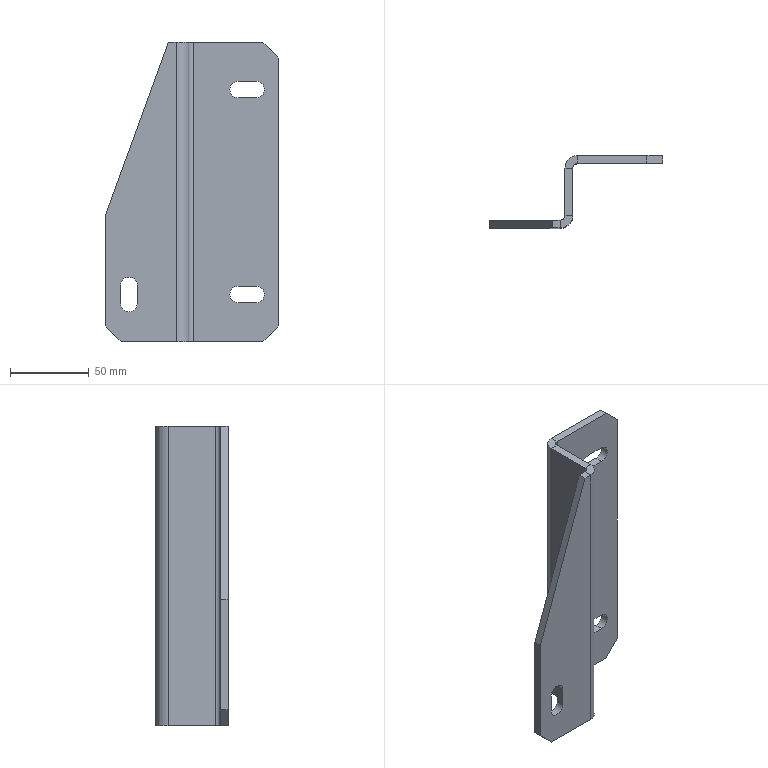Part | STEP file | PRT0001 | 1 solid | 41 faces | box 110 x 46 x 190 mm | volume 124105 mm3 | plane 28 | cylinder 13 | commonest cylinder face diameters 10.5 x9 6 x2 16 x2
STEP:
#1=CARTESIAN_POINT('',(-5.75,0.,124.75));
#2=VERTEX_POINT('',#1);
#3=CARTESIAN_POINT('',(5.75,0.,124.75));
#4=VERTEX_POINT('',#3);
#5=CARTESIAN_POINT('',(-5.75,0.,124.75));
#6=DIRECTION('',(1.,0.,0.));
#7=VECTOR('',#6,1000.);
#8=LINE('',#5,#7);
#9=EDGE_CURVE('',#2,#4,#8,.T.);
#10=ORIENTED_EDGE('',*,*,#9,.F.);
#11=CARTESIAN_POINT('',(-5.75,-5.,124.75));
#12=VERTEX_POINT('',#11);
#13=CARTESIAN_POINT('',(-5.75,-5.,124.75));
#14=DIRECTION('',(0.,1.,0.));
#15=VECTOR('',#14,1000.);
#16=LINE('',#13,#15);
#17=EDGE_CURVE('',#12,#2,#16,.T.);
#18=ORIENTED_EDGE('',*,*,#17,.F.);
#19=CARTESIAN_POINT('',(5.75,-5.,124.75));
#20=VERTEX_POINT('',#19);
#21=CARTESIAN_POINT('',(-5.75,-5.,124.75));
#22=DIRECTION('',(1.,0.,0.));
#23=VECTOR('',#22,1000.);
#24=LINE('',#21,#23);
#25=EDGE_CURVE('',#12,#20,#24,.T.);
#26=ORIENTED_EDGE('',*,*,#25,.T.);
#27=CARTESIAN_POINT('',(5.75,0.,124.75));
#28=DIRECTION('',(0.,-1.,0.));
#29=VECTOR('',#28,1000.);
#30=LINE('',#27,#29);
#31=EDGE_CURVE('',#4,#20,#30,.T.);
#32=ORIENTED_EDGE('',*,*,#31,.F.);
#33=EDGE_LOOP('',(#10,#18,#26,#32));
#34=FACE_OUTER_BOUND('',#33,.T.);
#35=CARTESIAN_POINT('',(-5.75,-10.,124.75));
#36=DIRECTION('',(0.,0.,-1.));
#37=DIRECTION('',(0.,-1.,0.));
#38=AXIS2_PLACEMENT_3D('',#35,#36,#37);
#39=PLANE('',#38);
#40=ADVANCED_FACE('',(#34),#39,.F.);
#41=CARTESIAN_POINT('',(5.75,-5.,135.25));
#42=VERTEX_POINT('',#41);
#43=CARTESIAN_POINT('',(5.75,0.,135.25));
#44=VERTEX_POINT('',#43);
#45=CARTESIAN_POINT('',(5.75,-5.,135.25));
#46=DIRECTION('',(0.,1.,0.));
#47=VECTOR('',#46,1000.);
#48=LINE('',#45,#47);
#49=EDGE_CURVE('',#42,#44,#48,.T.);
#50=ORIENTED_EDGE('',*,*,#49,.T.);
#51=CARTESIAN_POINT('',(5.75,0.,130.));
#52=DIRECTION('',(0.,-1.,0.));
#53=DIRECTION('',(0.,0.,-1.));
#54=AXIS2_PLACEMENT_3D('',#51,#52,#53);
#55=CIRCLE('',#54,5.25);
#56=EDGE_CURVE('',#4,#44,#55,.T.);
#57=ORIENTED_EDGE('',*,*,#56,.F.);
#58=ORIENTED_EDGE('',*,*,#31,.T.);
#59=CARTESIAN_POINT('',(5.75,-5.,130.));
#60=DIRECTION('',(0.,1.,0.));
#61=DIRECTION('',(0.,0.,1.));
#62=AXIS2_PLACEMENT_3D('',#59,#60,#61);
#63=CIRCLE('',#62,5.25);
#64=EDGE_CURVE('',#42,#20,#63,.T.);
#65=ORIENTED_EDGE('',*,*,#64,.F.);
#66=EDGE_LOOP('',(#50,#57,#58,#65));
#67=FACE_OUTER_BOUND('',#66,.T.);
#68=CARTESIAN_POINT('',(5.75,-10.,130.));
#69=DIRECTION('',(0.,1.,0.));
#70=DIRECTION('',(-1.,0.,0.));
#71=AXIS2_PLACEMENT_3D('',#68,#69,#70);
#72=CYLINDRICAL_SURFACE('',#71,5.25);
#73=ADVANCED_FACE('',(#67),#72,.F.);
#74=CARTESIAN_POINT('',(-5.75,0.,135.25));
#75=VERTEX_POINT('',#74);
#76=CARTESIAN_POINT('',(5.75,0.,135.25));
#77=DIRECTION('',(-1.,0.,0.));
#78=VECTOR('',#77,1000.);
#79=LINE('',#76,#78);
#80=EDGE_CURVE('',#44,#75,#79,.T.);
#81=ORIENTED_EDGE('',*,*,#80,.F.);
#82=ORIENTED_EDGE('',*,*,#49,.F.);
#83=CARTESIAN_POINT('',(-5.75,-5.,135.25));
#84=VERTEX_POINT('',#83);
#85=CARTESIAN_POINT('',(5.75,-5.,135.25));
#86=DIRECTION('',(-1.,0.,0.));
#87=VECTOR('',#86,1000.);
#88=LINE('',#85,#87);
#89=EDGE_CURVE('',#42,#84,#88,.T.);
#90=ORIENTED_EDGE('',*,*,#89,.T.);
#91=CARTESIAN_POINT('',(-5.75,0.,135.25));
#92=DIRECTION('',(0.,-1.,0.));
#93=VECTOR('',#92,1000.);
#94=LINE('',#91,#93);
#95=EDGE_CURVE('',#75,#84,#94,.T.);
#96=ORIENTED_EDGE('',*,*,#95,.F.);
#97=EDGE_LOOP('',(#81,#82,#90,#96));
#98=FACE_OUTER_BOUND('',#97,.T.);
#99=CARTESIAN_POINT('',(-5.75,-10.,135.25));
#100=DIRECTION('',(0.,0.,1.));
#101=DIRECTION('',(1.,0.,0.));
#102=AXIS2_PLACEMENT_3D('',#99,#100,#101);
#103=PLANE('',#102);
#104=ADVANCED_FACE('',(#98),#103,.F.);
#105=CARTESIAN_POINT('',(-11.,0.,130.));
#106=VERTEX_POINT('',#105);
#107=CARTESIAN_POINT('',(-11.,-5.,130.));
#108=VERTEX_POINT('',#107);
#109=CARTESIAN_POINT('',(-11.,0.,130.));
#110=DIRECTION('',(0.,-1.,0.));
#111=VECTOR('',#110,1000.);
#112=LINE('',#109,#111);
#113=EDGE_CURVE('',#106,#108,#112,.T.);
#114=ORIENTED_EDGE('',*,*,#113,.F.);
#115=CARTESIAN_POINT('',(-5.75,0.,130.));
#116=DIRECTION('',(0.,-1.,0.));
#117=DIRECTION('',(0.,0.,1.));
#118=AXIS2_PLACEMENT_3D('',#115,#116,#117);
#119=CIRCLE('',#118,5.25);
#120=EDGE_CURVE('',#75,#106,#119,.T.);
#121=ORIENTED_EDGE('',*,*,#120,.F.);
#122=ORIENTED_EDGE('',*,*,#95,.T.);
#123=CARTESIAN_POINT('',(-5.75,-5.,130.));
#124=DIRECTION('',(0.,1.,0.));
#125=DIRECTION('',(-1.,0.,0.));
#126=AXIS2_PLACEMENT_3D('',#123,#124,#125);
#127=CIRCLE('',#126,5.25);
#128=EDGE_CURVE('',#108,#84,#127,.T.);
#129=ORIENTED_EDGE('',*,*,#128,.F.);
#130=EDGE_LOOP('',(#114,#121,#122,#129));
#131=FACE_OUTER_BOUND('',#130,.T.);
#132=CARTESIAN_POINT('',(-5.75,-10.,130.));
#133=DIRECTION('',(0.,1.,0.));
#134=DIRECTION('',(-1.,0.,0.));
#135=AXIS2_PLACEMENT_3D('',#132,#133,#134);
#136=CYLINDRICAL_SURFACE('',#135,5.25);
#137=ADVANCED_FACE('',(#131),#136,.F.);
#138=CARTESIAN_POINT('',(-5.75,-5.,130.));
#139=DIRECTION('',(0.,1.,0.));
#140=DIRECTION('',(0.,0.,-1.));
#141=AXIS2_PLACEMENT_3D('',#138,#139,#140);
#142=CIRCLE('',#141,5.25);
#143=EDGE_CURVE('',#12,#108,#142,.T.);
#144=ORIENTED_EDGE('',*,*,#143,.F.);
#145=ORIENTED_EDGE('',*,*,#17,.T.);
#146=CARTESIAN_POINT('',(-5.75,0.,130.));
#147=DIRECTION('',(0.,-1.,0.));
#148=DIRECTION('',(-1.,0.,0.));
#149=AXIS2_PLACEMENT_3D('',#146,#147,#148);
#150=CIRCLE('',#149,5.25);
#151=EDGE_CURVE('',#106,#2,#150,.T.);
#152=ORIENTED_EDGE('',*,*,#151,.F.);
#153=ORIENTED_EDGE('',*,*,#113,.T.);
#154=EDGE_LOOP('',(#144,#145,#152,#153));
#155=FACE_OUTER_BOUND('',#154,.T.);
#156=CARTESIAN_POINT('',(-5.75,-10.,130.));
#157=DIRECTION('',(0.,1.,0.));
#158=DIRECTION('',(-1.,0.,0.));
#159=AXIS2_PLACEMENT_3D('',#156,#157,#158);
#160=CYLINDRICAL_SURFACE('',#159,5.25);
#161=ADVANCED_FACE('',(#155),#160,.F.);
#162=CARTESIAN_POINT('',(-5.75,0.,-5.25));
#163=VERTEX_POINT('',#162);
#164=CARTESIAN_POINT('',(5.75,0.,-5.25));
#165=VERTEX_POINT('',#164);
#166=CARTESIAN_POINT('',(-5.75,0.,-5.25));
#167=DIRECTION('',(1.,0.,0.));
#168=VECTOR('',#167,1000.);
#169=LINE('',#166,#168);
#170=EDGE_CURVE('',#163,#165,#169,.T.);
#171=ORIENTED_EDGE('',*,*,#170,.F.);
#172=CARTESIAN_POINT('',(-5.75,-5.,-5.25));
#173=VERTEX_POINT('',#172);
#174=CARTESIAN_POINT('',(-5.75,-5.,-5.25));
#175=DIRECTION('',(0.,1.,0.));
#176=VECTOR('',#175,1000.);
#177=LINE('',#174,#176);
#178=EDGE_CURVE('',#173,#163,#177,.T.);
#179=ORIENTED_EDGE('',*,*,#178,.F.);
#180=CARTESIAN_POINT('',(5.75,-5.,-5.25));
#181=VERTEX_POINT('',#180);
#182=CARTESIAN_POINT('',(-5.75,-5.,-5.25));
#183=DIRECTION('',(1.,0.,0.));
#184=VECTOR('',#183,1000.);
#185=LINE('',#182,#184);
#186=EDGE_CURVE('',#173,#181,#185,.T.);
#187=ORIENTED_EDGE('',*,*,#186,.T.);
#188=CARTESIAN_POINT('',(5.75,0.,-5.25));
#189=DIRECTION('',(0.,-1.,0.));
#190=VECTOR('',#189,1000.);
#191=LINE('',#188,#190);
#192=EDGE_CURVE('',#165,#181,#191,.T.);
#193=ORIENTED_EDGE('',*,*,#192,.F.);
#194=EDGE_LOOP('',(#171,#179,#187,#193));
#195=FACE_OUTER_BOUND('',#194,.T.);
#196=CARTESIAN_POINT('',(-5.75,-10.,-5.25));
#197=DIRECTION('',(0.,0.,-1.));
#198=DIRECTION('',(0.,-1.,0.));
#199=AXIS2_PLACEMENT_3D('',#196,#197,#198);
#200=PLANE('',#199);
#201=ADVANCED_FACE('',(#195),#200,.F.);
#202=CARTESIAN_POINT('',(5.75,-5.,5.25));
#203=VERTEX_POINT('',#202);
#204=CARTESIAN_POINT('',(5.75,0.,5.25));
#205=VERTEX_POINT('',#204);
#206=CARTESIAN_POINT('',(5.75,-5.,5.25));
#207=DIRECTION('',(0.,1.,0.));
#208=VECTOR('',#207,1000.);
#209=LINE('',#206,#208);
#210=EDGE_CURVE('',#203,#205,#209,.T.);
#211=ORIENTED_EDGE('',*,*,#210,.T.);
#212=CARTESIAN_POINT('',(5.75,0.,0.));
#213=DIRECTION('',(0.,-1.,0.));
#214=DIRECTION('',(0.,0.,-1.));
#215=AXIS2_PLACEMENT_3D('',#212,#213,#214);
#216=CIRCLE('',#215,5.25);
#217=EDGE_CURVE('',#165,#205,#216,.T.);
#218=ORIENTED_EDGE('',*,*,#217,.F.);
#219=ORIENTED_EDGE('',*,*,#192,.T.);
#220=CARTESIAN_POINT('',(5.75,-5.,0.));
#221=DIRECTION('',(0.,1.,0.));
#222=DIRECTION('',(0.,0.,1.));
#223=AXIS2_PLACEMENT_3D('',#220,#221,#222);
#224=CIRCLE('',#223,5.25);
#225=EDGE_CURVE('',#203,#181,#224,.T.);
#226=ORIENTED_EDGE('',*,*,#225,.F.);
#227=EDGE_LOOP('',(#211,#218,#219,#226));
#228=FACE_OUTER_BOUND('',#227,.T.);
#229=CARTESIAN_POINT('',(5.75,-10.,0.));
#230=DIRECTION('',(0.,1.,0.));
#231=DIRECTION('',(-1.,0.,0.));
#232=AXIS2_PLACEMENT_3D('',#229,#230,#231);
#233=CYLINDRICAL_SURFACE('',#232,5.25);
#234=ADVANCED_FACE('',(#228),#233,.F.);
#235=CARTESIAN_POINT('',(-5.75,0.,5.25));
#236=VERTEX_POINT('',#235);
#237=CARTESIAN_POINT('',(5.75,0.,5.25));
#238=DIRECTION('',(-1.,0.,0.));
#239=VECTOR('',#238,1000.);
#240=LINE('',#237,#239);
#241=EDGE_CURVE('',#205,#236,#240,.T.);
#242=ORIENTED_EDGE('',*,*,#241,.F.);
#243=ORIENTED_EDGE('',*,*,#210,.F.);
#244=CARTESIAN_POINT('',(-5.75,-5.,5.25));
#245=VERTEX_POINT('',#244);
#246=CARTESIAN_POINT('',(5.75,-5.,5.25));
#247=DIRECTION('',(-1.,0.,0.));
#248=VECTOR('',#247,1000.);
#249=LINE('',#246,#248);
#250=EDGE_CURVE('',#203,#245,#249,.T.);
#251=ORIENTED_EDGE('',*,*,#250,.T.);
#252=CARTESIAN_POINT('',(-5.75,0.,5.25));
#253=DIRECTION('',(0.,-1.,0.));
#254=VECTOR('',#253,1000.);
#255=LINE('',#252,#254);
#256=EDGE_CURVE('',#236,#245,#255,.T.);
#257=ORIENTED_EDGE('',*,*,#256,.F.);
#258=EDGE_LOOP('',(#242,#243,#251,#257));
#259=FACE_OUTER_BOUND('',#258,.T.);
#260=CARTESIAN_POINT('',(-5.75,-10.,5.25));
#261=DIRECTION('',(0.,0.,1.));
#262=DIRECTION('',(1.,0.,0.));
#263=AXIS2_PLACEMENT_3D('',#260,#261,#262);
#264=PLANE('',#263);
#265=ADVANCED_FACE('',(#259),#264,.F.);
#266=CARTESIAN_POINT('',(-11.,0.,0.));
#267=VERTEX_POINT('',#266);
#268=CARTESIAN_POINT('',(-11.,-5.,0.));
#269=VERTEX_POINT('',#268);
#270=CARTESIAN_POINT('',(-11.,0.,0.));
#271=DIRECTION('',(0.,-1.,0.));
#272=VECTOR('',#271,1000.);
#273=LINE('',#270,#272);
#274=EDGE_CURVE('',#267,#269,#273,.T.);
#275=ORIENTED_EDGE('',*,*,#274,.F.);
#276=CARTESIAN_POINT('',(-5.75,0.,0.));
#277=DIRECTION('',(0.,-1.,0.));
#278=DIRECTION('',(0.,0.,1.));
#279=AXIS2_PLACEMENT_3D('',#276,#277,#278);
#280=CIRCLE('',#279,5.25);
#281=EDGE_CURVE('',#236,#267,#280,.T.);
#282=ORIENTED_EDGE('',*,*,#281,.F.);
#283=ORIENTED_EDGE('',*,*,#256,.T.);
#284=CARTESIAN_POINT('',(-5.75,-5.,0.));
#285=DIRECTION('',(0.,1.,0.));
#286=DIRECTION('',(-1.,0.,0.));
#287=AXIS2_PLACEMENT_3D('',#284,#285,#286);
#288=CIRCLE('',#287,5.25);
#289=EDGE_CURVE('',#269,#245,#288,.T.);
#290=ORIENTED_EDGE('',*,*,#289,.F.);
#291=EDGE_LOOP('',(#275,#282,#283,#290));
#292=FACE_OUTER_BOUND('',#291,.T.);
#293=CARTESIAN_POINT('',(-5.75,-10.,0.));
#294=DIRECTION('',(0.,1.,0.));
#295=DIRECTION('',(-1.,0.,0.));
#296=AXIS2_PLACEMENT_3D('',#293,#294,#295);
#297=CYLINDRICAL_SURFACE('',#296,5.25);
#298=ADVANCED_FACE('',(#292),#297,.F.);
#299=CARTESIAN_POINT('',(-5.75,-5.,0.));
#300=DIRECTION('',(0.,1.,0.));
#301=DIRECTION('',(0.,0.,-1.));
#302=AXIS2_PLACEMENT_3D('',#299,#300,#301);
#303=CIRCLE('',#302,5.25);
#304=EDGE_CURVE('',#173,#269,#303,.T.);
#305=ORIENTED_EDGE('',*,*,#304,.F.);
#306=ORIENTED_EDGE('',*,*,#178,.T.);
#307=CARTESIAN_POINT('',(-5.75,0.,0.));
#308=DIRECTION('',(0.,-1.,0.));
#309=DIRECTION('',(-1.,0.,0.));
#310=AXIS2_PLACEMENT_3D('',#307,#308,#309);
#311=CIRCLE('',#310,5.25);
#312=EDGE_CURVE('',#267,#163,#311,.T.);
#313=ORIENTED_EDGE('',*,*,#312,.F.);
#314=ORIENTED_EDGE('',*,*,#274,.T.);
#315=EDGE_LOOP('',(#305,#306,#313,#314));
#316=FACE_OUTER_BOUND('',#315,.T.);
#317=CARTESIAN_POINT('',(-5.75,-10.,0.));
#318=DIRECTION('',(0.,1.,0.));
#319=DIRECTION('',(-1.,0.,0.));
#320=AXIS2_PLACEMENT_3D('',#317,#318,#319);
#321=CYLINDRICAL_SURFACE('',#320,5.25);
#322=ADVANCED_FACE('',(#316),#321,.F.);
#323=CARTESIAN_POINT('',(20.,0.,-20.));
#324=VERTEX_POINT('',#323);
#325=CARTESIAN_POINT('',(20.,-5.,-20.));
#326=VERTEX_POINT('',#325);
#327=CARTESIAN_POINT('',(20.,0.,-20.));
#328=DIRECTION('',(0.,-1.,0.));
#329=VECTOR('',#328,1000.);
#330=LINE('',#327,#329);
#331=EDGE_CURVE('',#324,#326,#330,.T.);
#332=ORIENTED_EDGE('',*,*,#331,.T.);
#333=CARTESIAN_POINT('',(10.,-5.,-30.));
#334=VERTEX_POINT('',#333);
#335=CARTESIAN_POINT('',(10.,-5.,-30.));
#336=DIRECTION('',(0.7071,0.,0.7071));
#337=VECTOR('',#336,1000.);
#338=LINE('',#335,#337);
#339=EDGE_CURVE('',#334,#326,#338,.T.);
#340=ORIENTED_EDGE('',*,*,#339,.F.);
#341=CARTESIAN_POINT('',(10.,0.,-30.));
#342=VERTEX_POINT('',#341);
#343=CARTESIAN_POINT('',(10.,-5.,-30.));
#344=DIRECTION('',(0.,1.,0.));
#345=VECTOR('',#344,1000.);
#346=LINE('',#343,#345);
#347=EDGE_CURVE('',#334,#342,#346,.T.);
#348=ORIENTED_EDGE('',*,*,#347,.T.);
#349=CARTESIAN_POINT('',(20.,0.,-20.));
#350=DIRECTION('',(-0.7071,0.,-0.7071));
#351=VECTOR('',#350,1000.);
#352=LINE('',#349,#351);
#353=EDGE_CURVE('',#324,#342,#352,.T.);
#354=ORIENTED_EDGE('',*,*,#353,.F.);
#355=EDGE_LOOP('',(#332,#340,#348,#354));
#356=FACE_OUTER_BOUND('',#355,.T.);
#357=CARTESIAN_POINT('',(10.,-8.,-30.));
#358=DIRECTION('',(0.7071,0.,-0.7071));
#359=DIRECTION('',(0.,-1.,0.));
#360=AXIS2_PLACEMENT_3D('',#357,#358,#359);
#361=PLANE('',#360);
#362=ADVANCED_FACE('',(#356),#361,.T.);
#363=CARTESIAN_POINT('',(-80.25,-41.,5.75));
#364=VERTEX_POINT('',#363);
#365=CARTESIAN_POINT('',(-80.25,-41.,-5.75));
#366=VERTEX_POINT('',#365);
#367=CARTESIAN_POINT('',(-80.25,-41.,5.75));
#368=DIRECTION('',(0.,0.,-1.));
#369=VECTOR('',#368,1000.);
#370=LINE('',#367,#369);
#371=EDGE_CURVE('',#364,#366,#370,.T.);
#372=ORIENTED_EDGE('',*,*,#371,.F.);
#373=CARTESIAN_POINT('',(-80.25,-46.,5.75));
#374=VERTEX_POINT('',#373);
#375=CARTESIAN_POINT('',(-80.25,-46.,5.75));
#376=DIRECTION('',(0.,1.,0.));
#377=VECTOR('',#376,1000.);
#378=LINE('',#375,#377);
#379=EDGE_CURVE('',#374,#364,#378,.T.);
#380=ORIENTED_EDGE('',*,*,#379,.F.);
#381=CARTESIAN_POINT('',(-80.25,-46.,-5.75));
#382=VERTEX_POINT('',#381);
#383=CARTESIAN_POINT('',(-80.25,-46.,5.75));
#384=DIRECTION('',(0.,0.,-1.));
#385=VECTOR('',#384,1000.);
#386=LINE('',#383,#385);
#387=EDGE_CURVE('',#374,#382,#386,.T.);
#388=ORIENTED_EDGE('',*,*,#387,.T.);
#389=CARTESIAN_POINT('',(-80.25,-41.,-5.75));
#390=DIRECTION('',(0.,-1.,0.));
#391=VECTOR('',#390,1000.);
#392=LINE('',#389,#391);
#393=EDGE_CURVE('',#366,#382,#392,.T.);
#394=ORIENTED_EDGE('',*,*,#393,.F.);
#395=EDGE_LOOP('',(#372,#380,#388,#394));
#396=FACE_OUTER_BOUND('',#395,.T.);
#397=CARTESIAN_POINT('',(-80.25,-51.,5.75));
#398=DIRECTION('',(-1.,0.,0.));
#399=DIRECTION('',(0.,0.,1.));
#400=AXIS2_PLACEMENT_3D('',#397,#398,#399);
#401=PLANE('',#400);
#402=ADVANCED_FACE('',(#396),#401,.F.);
#403=CARTESIAN_POINT('',(-69.75,-46.,-5.75));
#404=VERTEX_POINT('',#403);
#405=CARTESIAN_POINT('',(-69.75,-41.,-5.75));
#406=VERTEX_POINT('',#405);
#407=CARTESIAN_POINT('',(-69.75,-46.,-5.75));
#408=DIRECTION('',(0.,1.,0.));
#409=VECTOR('',#408,1000.);
#410=LINE('',#407,#409);
#411=EDGE_CURVE('',#404,#406,#410,.T.);
#412=ORIENTED_EDGE('',*,*,#411,.T.);
#413=CARTESIAN_POINT('',(-75.,-41.,-5.75));
#414=DIRECTION('',(0.,-1.,0.));
#415=DIRECTION('',(-1.,0.,0.));
#416=AXIS2_PLACEMENT_3D('',#413,#414,#415);
#417=CIRCLE('',#416,5.25);
#418=EDGE_CURVE('',#366,#406,#417,.T.);
#419=ORIENTED_EDGE('',*,*,#418,.F.);
#420=ORIENTED_EDGE('',*,*,#393,.T.);
#421=CARTESIAN_POINT('',(-75.,-46.,-5.75));
#422=DIRECTION('',(0.,1.,0.));
#423=DIRECTION('',(1.,0.,0.));
#424=AXIS2_PLACEMENT_3D('',#421,#422,#423);
#425=CIRCLE('',#424,5.25);
#426=EDGE_CURVE('',#404,#382,#425,.T.);
#427=ORIENTED_EDGE('',*,*,#426,.F.);
#428=EDGE_LOOP('',(#412,#419,#420,#427));
#429=FACE_OUTER_BOUND('',#428,.T.);
#430=CARTESIAN_POINT('',(-75.,-51.,-5.75));
#431=DIRECTION('',(0.,1.,0.));
#432=DIRECTION('',(0.,0.,1.));
#433=AXIS2_PLACEMENT_3D('',#430,#431,#432);
#434=CYLINDRICAL_SURFACE('',#433,5.25);
#435=ADVANCED_FACE('',(#429),#434,.F.);
#436=CARTESIAN_POINT('',(-69.75,-41.,5.75));
#437=VERTEX_POINT('',#436);
#438=CARTESIAN_POINT('',(-69.75,-41.,-5.75));
#439=DIRECTION('',(0.,0.,1.));
#440=VECTOR('',#439,1000.);
#441=LINE('',#438,#440);
#442=EDGE_CURVE('',#406,#437,#441,.T.);
#443=ORIENTED_EDGE('',*,*,#442,.F.);
#444=ORIENTED_EDGE('',*,*,#411,.F.);
#445=CARTESIAN_POINT('',(-69.75,-46.,5.75));
#446=VERTEX_POINT('',#445);
#447=CARTESIAN_POINT('',(-69.75,-46.,-5.75));
#448=DIRECTION('',(0.,0.,1.));
#449=VECTOR('',#448,1000.);
#450=LINE('',#447,#449);
#451=EDGE_CURVE('',#404,#446,#450,.T.);
#452=ORIENTED_EDGE('',*,*,#451,.T.);
#453=CARTESIAN_POINT('',(-69.75,-41.,5.75));
#454=DIRECTION('',(0.,-1.,0.));
#455=VECTOR('',#454,1000.);
#456=LINE('',#453,#455);
#457=EDGE_CURVE('',#437,#446,#456,.T.);
#458=ORIENTED_EDGE('',*,*,#457,.F.);
#459=EDGE_LOOP('',(#443,#444,#452,#458));
#460=FACE_OUTER_BOUND('',#459,.T.);
#461=CARTESIAN_POINT('',(-69.75,-51.,5.75));
#462=DIRECTION('',(1.,0.,0.));
#463=DIRECTION('',(0.,1.,0.));
#464=AXIS2_PLACEMENT_3D('',#461,#462,#463);
#465=PLANE('',#464);
#466=ADVANCED_FACE('',(#460),#465,.F.);
#467=CARTESIAN_POINT('',(-75.,-41.,11.));
#468=VERTEX_POINT('',#467);
#469=CARTESIAN_POINT('',(-75.,-46.,11.));
#470=VERTEX_POINT('',#469);
#471=CARTESIAN_POINT('',(-75.,-41.,11.));
#472=DIRECTION('',(0.,-1.,0.));
#473=VECTOR('',#472,1000.);
#474=LINE('',#471,#473);
#475=EDGE_CURVE('',#468,#470,#474,.T.);
#476=ORIENTED_EDGE('',*,*,#475,.F.);
#477=CARTESIAN_POINT('',(-75.,-41.,5.75));
#478=DIRECTION('',(0.,-1.,0.));
#479=DIRECTION('',(1.,0.,0.));
#480=AXIS2_PLACEMENT_3D('',#477,#478,#479);
#481=CIRCLE('',#480,5.25);
#482=EDGE_CURVE('',#437,#468,#481,.T.);
#483=ORIENTED_EDGE('',*,*,#482,.F.);
#484=ORIENTED_EDGE('',*,*,#457,.T.);
#485=CARTESIAN_POINT('',(-75.,-46.,5.75));
#486=DIRECTION('',(0.,1.,0.));
#487=DIRECTION('',(0.,0.,1.));
#488=AXIS2_PLACEMENT_3D('',#485,#486,#487);
#489=CIRCLE('',#488,5.25);
#490=EDGE_CURVE('',#470,#446,#489,.T.);
#491=ORIENTED_EDGE('',*,*,#490,.F.);
#492=EDGE_LOOP('',(#476,#483,#484,#491));
#493=FACE_OUTER_BOUND('',#492,.T.);
#494=CARTESIAN_POINT('',(-75.,-51.,5.75));
#495=DIRECTION('',(0.,1.,0.));
#496=DIRECTION('',(0.,0.,1.));
#497=AXIS2_PLACEMENT_3D('',#494,#495,#496);
#498=CYLINDRICAL_SURFACE('',#497,5.25);
#499=ADVANCED_FACE('',(#493),#498,.F.);
#500=CARTESIAN_POINT('',(-75.,-46.,5.75));
#501=DIRECTION('',(0.,1.,0.));
#502=DIRECTION('',(-1.,0.,0.));
#503=AXIS2_PLACEMENT_3D('',#500,#501,#502);
#504=CIRCLE('',#503,5.25);
#505=EDGE_CURVE('',#374,#470,#504,.T.);
#506=ORIENTED_EDGE('',*,*,#505,.F.);
#507=ORIENTED_EDGE('',*,*,#379,.T.);
#508=CARTESIAN_POINT('',(-75.,-41.,5.75));
#509=DIRECTION('',(0.,-1.,0.));
#510=DIRECTION('',(0.,0.,1.));
#511=AXIS2_PLACEMENT_3D('',#508,#509,#510);
#512=CIRCLE('',#511,5.25);
#513=EDGE_CURVE('',#468,#364,#512,.T.);
#514=ORIENTED_EDGE('',*,*,#513,.F.);
#515=ORIENTED_EDGE('',*,*,#475,.T.);
#516=EDGE_LOOP('',(#506,#507,#514,#515));
#517=FACE_OUTER_BOUND('',#516,.T.);
#518=CARTESIAN_POINT('',(-75.,-51.,5.75));
#519=DIRECTION('',(0.,1.,0.));
#520=DIRECTION('',(0.,0.,1.));
#521=AXIS2_PLACEMENT_3D('',#518,#519,#520);
#522=CYLINDRICAL_SURFACE('',#521,5.25);
#523=ADVANCED_FACE('',(#517),#522,.F.);
#524=CARTESIAN_POINT('',(-90.,-46.,-20.));
#525=VERTEX_POINT('',#524);
#526=CARTESIAN_POINT('',(-90.,-41.,-20.));
#527=VERTEX_POINT('',#526);
#528=CARTESIAN_POINT('',(-90.,-46.,-20.));
#529=DIRECTION('',(0.,1.,0.));
#530=VECTOR('',#529,1000.);
#531=LINE('',#528,#530);
#532=EDGE_CURVE('',#525,#527,#531,.T.);
#533=ORIENTED_EDGE('',*,*,#532,.T.);
#534=CARTESIAN_POINT('',(-80.,-41.,-30.));
#535=VERTEX_POINT('',#534);
#536=CARTESIAN_POINT('',(-80.,-41.,-30.));
#537=DIRECTION('',(-0.7071,0.,0.7071));
#538=VECTOR('',#537,1000.);
#539=LINE('',#536,#538);
#540=EDGE_CURVE('',#535,#527,#539,.T.);
#541=ORIENTED_EDGE('',*,*,#540,.F.);
#542=CARTESIAN_POINT('',(-80.,-46.,-30.));
#543=VERTEX_POINT('',#542);
#544=CARTESIAN_POINT('',(-80.,-41.,-30.));
#545=DIRECTION('',(0.,-1.,0.));
#546=VECTOR('',#545,1000.);
#547=LINE('',#544,#546);
#548=EDGE_CURVE('',#535,#543,#547,.T.);
#549=ORIENTED_EDGE('',*,*,#548,.T.);
#550=CARTESIAN_POINT('',(-90.,-46.,-20.));
#551=DIRECTION('',(0.7071,0.,-0.7071));
#552=VECTOR('',#551,1000.);
#553=LINE('',#550,#552);
#554=EDGE_CURVE('',#525,#543,#553,.T.);
#555=ORIENTED_EDGE('',*,*,#554,.F.);
#556=EDGE_LOOP('',(#533,#541,#549,#555));
#557=FACE_OUTER_BOUND('',#556,.T.);
#558=CARTESIAN_POINT('',(-80.,-38.,-30.));
#559=DIRECTION('',(0.7071,0.,0.7071));
#560=DIRECTION('',(0.,-1.,0.));
#561=AXIS2_PLACEMENT_3D('',#558,#559,#560);
#562=PLANE('',#561);
#563=ADVANCED_FACE('',(#557),#562,.F.);
#564=CARTESIAN_POINT('',(-90.,-41.,50.));
#565=VERTEX_POINT('',#564);
#566=CARTESIAN_POINT('',(-90.,-41.,-20.));
#567=DIRECTION('',(0.,0.,1.));
#568=VECTOR('',#567,1000.);
#569=LINE('',#566,#568);
#570=EDGE_CURVE('',#527,#565,#569,.T.);
#571=ORIENTED_EDGE('',*,*,#570,.F.);
#572=ORIENTED_EDGE('',*,*,#532,.F.);
#573=CARTESIAN_POINT('',(-90.,-46.,50.));
#574=VERTEX_POINT('',#573);
#575=CARTESIAN_POINT('',(-90.,-46.,-20.));
#576=DIRECTION('',(0.,0.,1.));
#577=VECTOR('',#576,1000.);
#578=LINE('',#575,#577);
#579=EDGE_CURVE('',#525,#574,#578,.T.);
#580=ORIENTED_EDGE('',*,*,#579,.T.);
#581=CARTESIAN_POINT('',(-90.,-41.,50.));
#582=DIRECTION('',(0.,-1.,0.));
#583=VECTOR('',#582,1000.);
#584=LINE('',#581,#583);
#585=EDGE_CURVE('',#565,#574,#584,.T.);
#586=ORIENTED_EDGE('',*,*,#585,.F.);
#587=EDGE_LOOP('',(#571,#572,#580,#586));
#588=FACE_OUTER_BOUND('',#587,.T.);
#589=CARTESIAN_POINT('',(-90.,-46.,160.));
#590=DIRECTION('',(-1.,0.,0.));
#591=DIRECTION('',(0.,0.,1.));
#592=AXIS2_PLACEMENT_3D('',#589,#590,#591);
#593=PLANE('',#592);
#594=ADVANCED_FACE('',(#588),#593,.T.);
#595=ORIENTED_EDGE('',*,*,#371,.T.);
#596=ORIENTED_EDGE('',*,*,#418,.T.);
#597=ORIENTED_EDGE('',*,*,#442,.T.);
#598=ORIENTED_EDGE('',*,*,#482,.T.);
#599=ORIENTED_EDGE('',*,*,#513,.T.);
#600=EDGE_LOOP('',(#595,#596,#597,#598,#599));
#601=FACE_BOUND('',#600,.T.);
#602=CARTESIAN_POINT('',(-45.,-41.,160.));
#603=VERTEX_POINT('',#602);
#604=CARTESIAN_POINT('',(-50.,-41.,160.));
#605=VERTEX_POINT('',#604);
#606=CARTESIAN_POINT('',(-45.,-41.,160.));
#607=DIRECTION('',(-1.,0.,0.));
#608=VECTOR('',#607,1000.);
#609=LINE('',#606,#608);
#610=EDGE_CURVE('',#603,#605,#609,.T.);
#611=ORIENTED_EDGE('',*,*,#610,.F.);
#612=CARTESIAN_POINT('',(-45.,-41.,-30.));
#613=VERTEX_POINT('',#612);
#614=CARTESIAN_POINT('',(-45.,-41.,-30.));
#615=DIRECTION('',(0.,0.,1.));
#616=VECTOR('',#615,1000.);
#617=LINE('',#614,#616);
#618=EDGE_CURVE('',#613,#603,#617,.T.);
#619=ORIENTED_EDGE('',*,*,#618,.F.);
#620=CARTESIAN_POINT('',(-45.,-41.,-30.));
#621=DIRECTION('',(-1.,0.,0.));
#622=VECTOR('',#621,1000.);
#623=LINE('',#620,#622);
#624=EDGE_CURVE('',#613,#535,#623,.T.);
#625=ORIENTED_EDGE('',*,*,#624,.T.);
#626=ORIENTED_EDGE('',*,*,#540,.T.);
#627=ORIENTED_EDGE('',*,*,#570,.T.);
#628=CARTESIAN_POINT('',(-90.,-41.,50.));
#629=DIRECTION('',(0.3417,0.,0.9398));
#630=VECTOR('',#629,1000.);
#631=LINE('',#628,#630);
#632=EDGE_CURVE('',#565,#605,#631,.T.);
#633=ORIENTED_EDGE('',*,*,#632,.T.);
#634=EDGE_LOOP('',(#611,#619,#625,#626,#627,#633));
#635=FACE_OUTER_BOUND('',#634,.T.);
#636=CARTESIAN_POINT('',(-90.,-41.,160.));
#637=DIRECTION('',(0.,1.,0.));
#638=DIRECTION('',(1.,0.,0.));
#639=AXIS2_PLACEMENT_3D('',#636,#637,#638);
#640=PLANE('',#639);
#641=ADVANCED_FACE('',(#601,#635),#640,.T.);
#642=ORIENTED_EDGE('',*,*,#548,.F.);
#643=ORIENTED_EDGE('',*,*,#624,.F.);
#644=CARTESIAN_POINT('',(-45.,-46.,-30.));
#645=VERTEX_POINT('',#644);
#646=CARTESIAN_POINT('',(-45.,-46.,-30.));
#647=DIRECTION('',(0.,1.,0.));
#648=VECTOR('',#647,1000.);
#649=LINE('',#646,#648);
#650=EDGE_CURVE('',#645,#613,#649,.T.);
#651=ORIENTED_EDGE('',*,*,#650,.F.);
#652=CARTESIAN_POINT('',(-45.,-46.,-30.));
#653=DIRECTION('',(-1.,0.,0.));
#654=VECTOR('',#653,1000.);
#655=LINE('',#652,#654);
#656=EDGE_CURVE('',#645,#543,#655,.T.);
#657=ORIENTED_EDGE('',*,*,#656,.T.);
#658=EDGE_LOOP('',(#642,#643,#651,#657));
#659=FACE_OUTER_BOUND('',#658,.T.);
#660=CARTESIAN_POINT('',(-37.,-38.,-30.));
#661=DIRECTION('',(0.,0.,-1.));
#662=DIRECTION('',(0.,-1.,0.));
#663=AXIS2_PLACEMENT_3D('',#660,#661,#662);
#664=PLANE('',#663);
#665=ADVANCED_FACE('',(#659),#664,.T.);
#666=ORIENTED_EDGE('',*,*,#505,.T.);
#667=ORIENTED_EDGE('',*,*,#490,.T.);
#668=ORIENTED_EDGE('',*,*,#451,.F.);
#669=ORIENTED_EDGE('',*,*,#426,.T.);
#670=ORIENTED_EDGE('',*,*,#387,.F.);
#671=EDGE_LOOP('',(#666,#667,#668,#669,#670));
#672=FACE_BOUND('',#671,.T.);
#673=CARTESIAN_POINT('',(-50.,-46.,160.));
#674=VERTEX_POINT('',#673);
#675=CARTESIAN_POINT('',(-50.,-46.,160.));
#676=DIRECTION('',(-0.3417,0.,-0.9398));
#677=VECTOR('',#676,1000.);
#678=LINE('',#675,#677);
#679=EDGE_CURVE('',#674,#574,#678,.T.);
#680=ORIENTED_EDGE('',*,*,#679,.T.);
#681=ORIENTED_EDGE('',*,*,#579,.F.);
#682=ORIENTED_EDGE('',*,*,#554,.T.);
#683=ORIENTED_EDGE('',*,*,#656,.F.);
#684=CARTESIAN_POINT('',(-45.,-46.,160.));
#685=VERTEX_POINT('',#684);
#686=CARTESIAN_POINT('',(-45.,-46.,160.));
#687=DIRECTION('',(0.,0.,-1.));
#688=VECTOR('',#687,1000.);
#689=LINE('',#686,#688);
#690=EDGE_CURVE('',#685,#645,#689,.T.);
#691=ORIENTED_EDGE('',*,*,#690,.F.);
#692=CARTESIAN_POINT('',(-45.,-46.,160.));
#693=DIRECTION('',(-1.,0.,0.));
#694=VECTOR('',#693,1000.);
#695=LINE('',#692,#694);
#696=EDGE_CURVE('',#685,#674,#695,.T.);
#697=ORIENTED_EDGE('',*,*,#696,.T.);
#698=EDGE_LOOP('',(#680,#681,#682,#683,#691,#697));
#699=FACE_OUTER_BOUND('',#698,.T.);
#700=CARTESIAN_POINT('',(-90.,-46.,160.));
#701=DIRECTION('',(0.,1.,0.));
#702=DIRECTION('',(1.,0.,0.));
#703=AXIS2_PLACEMENT_3D('',#700,#701,#702);
#704=PLANE('',#703);
#705=ADVANCED_FACE('',(#672,#699),#704,.F.);
#706=ORIENTED_EDGE('',*,*,#632,.F.);
#707=ORIENTED_EDGE('',*,*,#585,.T.);
#708=ORIENTED_EDGE('',*,*,#679,.F.);
#709=CARTESIAN_POINT('',(-50.,-41.,160.));
#710=DIRECTION('',(0.,-1.,0.));
#711=VECTOR('',#710,1000.);
#712=LINE('',#709,#711);
#713=EDGE_CURVE('',#605,#674,#712,.T.);
#714=ORIENTED_EDGE('',*,*,#713,.F.);
#715=EDGE_LOOP('',(#706,#707,#708,#714));
#716=FACE_OUTER_BOUND('',#715,.T.);
#717=CARTESIAN_POINT('',(-90.,-51.,50.));
#718=DIRECTION('',(0.9398,0.,-0.3417));
#719=DIRECTION('',(0.,-1.,0.));
#720=AXIS2_PLACEMENT_3D('',#717,#718,#719);
#721=PLANE('',#720);
#722=ADVANCED_FACE('',(#716),#721,.F.);
#723=ORIENTED_EDGE('',*,*,#696,.F.);
#724=CARTESIAN_POINT('',(-45.,-41.,160.));
#725=DIRECTION('',(0.,-1.,0.));
#726=VECTOR('',#725,1000.);
#727=LINE('',#724,#726);
#728=EDGE_CURVE('',#603,#685,#727,.T.);
#729=ORIENTED_EDGE('',*,*,#728,.F.);
#730=ORIENTED_EDGE('',*,*,#610,.T.);
#731=ORIENTED_EDGE('',*,*,#713,.T.);
#732=EDGE_LOOP('',(#723,#729,#730,#731));
#733=FACE_OUTER_BOUND('',#732,.T.);
#734=CARTESIAN_POINT('',(-34.,-8.,160.));
#735=DIRECTION('',(0.,0.,1.));
#736=DIRECTION('',(1.,0.,0.));
#737=AXIS2_PLACEMENT_3D('',#734,#735,#736);
#738=PLANE('',#737);
#739=ADVANCED_FACE('',(#733),#738,.T.);
#740=CARTESIAN_POINT('',(-37.,-38.,160.));
#741=VERTEX_POINT('',#740);
#742=CARTESIAN_POINT('',(-45.,-38.,160.));
#743=DIRECTION('',(0.,0.,1.));
#744=DIRECTION('',(0.,-1.,0.));
#745=AXIS2_PLACEMENT_3D('',#742,#743,#744);
#746=CIRCLE('',#745,8.);
#747=EDGE_CURVE('',#685,#741,#746,.T.);
#748=ORIENTED_EDGE('',*,*,#747,.T.);
#749=CARTESIAN_POINT('',(-42.,-38.,160.));
#750=VERTEX_POINT('',#749);
#751=CARTESIAN_POINT('',(-37.,-38.,160.));
#752=DIRECTION('',(-1.,0.,0.));
#753=VECTOR('',#752,1000.);
#754=LINE('',#751,#753);
#755=EDGE_CURVE('',#741,#750,#754,.T.);
#756=ORIENTED_EDGE('',*,*,#755,.T.);
#757=CARTESIAN_POINT('',(-45.,-38.,160.));
#758=DIRECTION('',(0.,0.,-1.));
#759=DIRECTION('',(1.,0.,0.));
#760=AXIS2_PLACEMENT_3D('',#757,#758,#759);
#761=CIRCLE('',#760,3.);
#762=EDGE_CURVE('',#750,#603,#761,.T.);
#763=ORIENTED_EDGE('',*,*,#762,.T.);
#764=ORIENTED_EDGE('',*,*,#728,.T.);
#765=EDGE_LOOP('',(#748,#756,#763,#764));
#766=FACE_OUTER_BOUND('',#765,.T.);
#767=CARTESIAN_POINT('',(-45.,-38.,160.));
#768=DIRECTION('',(0.,0.,-1.));
#769=DIRECTION('',(0.,-1.,0.));
#770=AXIS2_PLACEMENT_3D('',#767,#768,#769);
#771=PLANE('',#770);
#772=ADVANCED_FACE('',(#766),#771,.F.);
#773=CARTESIAN_POINT('',(-42.,-38.,-30.));
#774=VERTEX_POINT('',#773);
#775=CARTESIAN_POINT('',(-45.,-38.,-30.));
#776=DIRECTION('',(0.,0.,1.));
#777=DIRECTION('',(0.,-1.,0.));
#778=AXIS2_PLACEMENT_3D('',#775,#776,#777);
#779=CIRCLE('',#778,3.);
#780=EDGE_CURVE('',#613,#774,#779,.T.);
#781=ORIENTED_EDGE('',*,*,#780,.F.);
#782=ORIENTED_EDGE('',*,*,#618,.T.);
#783=ORIENTED_EDGE('',*,*,#762,.F.);
#784=CARTESIAN_POINT('',(-42.,-38.,160.));
#785=DIRECTION('',(0.,0.,-1.));
#786=VECTOR('',#785,1000.);
#787=LINE('',#784,#786);
#788=EDGE_CURVE('',#750,#774,#787,.T.);
#789=ORIENTED_EDGE('',*,*,#788,.T.);
#790=EDGE_LOOP('',(#781,#782,#783,#789));
#791=FACE_OUTER_BOUND('',#790,.T.);
#792=CARTESIAN_POINT('',(-45.,-38.,-125.195));
#793=DIRECTION('',(0.,0.,1.));
#794=DIRECTION('',(1.,0.,0.));
#795=AXIS2_PLACEMENT_3D('',#792,#793,#794);
#796=CYLINDRICAL_SURFACE('',#795,3.);
#797=ADVANCED_FACE('',(#791),#796,.F.);
#798=CARTESIAN_POINT('',(-37.,-8.,-30.));
#799=VERTEX_POINT('',#798);
#800=CARTESIAN_POINT('',(-42.,-8.,-30.));
#801=VERTEX_POINT('',#800);
#802=CARTESIAN_POINT('',(-37.,-8.,-30.));
#803=DIRECTION('',(-1.,0.,0.));
#804=VECTOR('',#803,1000.);
#805=LINE('',#802,#804);
#806=EDGE_CURVE('',#799,#801,#805,.T.);
#807=ORIENTED_EDGE('',*,*,#806,.F.);
#808=CARTESIAN_POINT('',(-37.,-38.,-30.));
#809=VERTEX_POINT('',#808);
#810=CARTESIAN_POINT('',(-37.,-8.,-30.));
#811=DIRECTION('',(0.,-1.,0.));
#812=VECTOR('',#811,1000.);
#813=LINE('',#810,#812);
#814=EDGE_CURVE('',#799,#809,#813,.T.);
#815=ORIENTED_EDGE('',*,*,#814,.T.);
#816=CARTESIAN_POINT('',(-42.,-38.,-30.));
#817=DIRECTION('',(1.,0.,0.));
#818=VECTOR('',#817,1000.);
#819=LINE('',#816,#818);
#820=EDGE_CURVE('',#774,#809,#819,.T.);
#821=ORIENTED_EDGE('',*,*,#820,.F.);
#822=CARTESIAN_POINT('',(-42.,-8.,-30.));
#823=DIRECTION('',(0.,-1.,0.));
#824=VECTOR('',#823,1000.);
#825=LINE('',#822,#824);
#826=EDGE_CURVE('',#801,#774,#825,.T.);
#827=ORIENTED_EDGE('',*,*,#826,.F.);
#828=EDGE_LOOP('',(#807,#815,#821,#827));
#829=FACE_OUTER_BOUND('',#828,.T.);
#830=CARTESIAN_POINT('',(-34.,-5.,-30.));
#831=DIRECTION('',(0.,0.,-1.));
#832=DIRECTION('',(0.,-1.,0.));
#833=AXIS2_PLACEMENT_3D('',#830,#831,#832);
#834=PLANE('',#833);
#835=ADVANCED_FACE('',(#829),#834,.T.);
#836=ORIENTED_EDGE('',*,*,#650,.T.);
#837=ORIENTED_EDGE('',*,*,#780,.T.);
#838=ORIENTED_EDGE('',*,*,#820,.T.);
#839=CARTESIAN_POINT('',(-45.,-38.,-30.));
#840=DIRECTION('',(0.,0.,-1.));
#841=DIRECTION('',(1.,0.,0.));
#842=AXIS2_PLACEMENT_3D('',#839,#840,#841);
#843=CIRCLE('',#842,8.);
#844=EDGE_CURVE('',#809,#645,#843,.T.);
#845=ORIENTED_EDGE('',*,*,#844,.T.);
#846=EDGE_LOOP('',(#836,#837,#838,#845));
#847=FACE_OUTER_BOUND('',#846,.T.);
#848=CARTESIAN_POINT('',(-45.,-38.,-30.));
#849=DIRECTION('',(0.,0.,1.));
#850=DIRECTION('',(1.,0.,0.));
#851=AXIS2_PLACEMENT_3D('',#848,#849,#850);
#852=PLANE('',#851);
#853=ADVANCED_FACE('',(#847),#852,.F.);
#854=ORIENTED_EDGE('',*,*,#747,.F.);
#855=ORIENTED_EDGE('',*,*,#690,.T.);
#856=ORIENTED_EDGE('',*,*,#844,.F.);
#857=CARTESIAN_POINT('',(-37.,-38.,-30.));
#858=DIRECTION('',(0.,0.,1.));
#859=VECTOR('',#858,1000.);
#860=LINE('',#857,#859);
#861=EDGE_CURVE('',#809,#741,#860,.T.);
#862=ORIENTED_EDGE('',*,*,#861,.T.);
#863=EDGE_LOOP('',(#854,#855,#856,#862));
#864=FACE_OUTER_BOUND('',#863,.T.);
#865=CARTESIAN_POINT('',(-45.,-38.,-125.195));
#866=DIRECTION('',(0.,0.,1.));
#867=DIRECTION('',(1.,0.,0.));
#868=AXIS2_PLACEMENT_3D('',#865,#866,#867);
#869=CYLINDRICAL_SURFACE('',#868,8.);
#870=ADVANCED_FACE('',(#864),#869,.T.);
#871=ORIENTED_EDGE('',*,*,#814,.F.);
#872=CARTESIAN_POINT('',(-37.,-8.,160.));
#873=VERTEX_POINT('',#872);
#874=CARTESIAN_POINT('',(-37.,-8.,160.));
#875=DIRECTION('',(0.,0.,-1.));
#876=VECTOR('',#875,1000.);
#877=LINE('',#874,#876);
#878=EDGE_CURVE('',#873,#799,#877,.T.);
#879=ORIENTED_EDGE('',*,*,#878,.F.);
#880=CARTESIAN_POINT('',(-37.,-8.,160.));
#881=DIRECTION('',(0.,-1.,0.));
#882=VECTOR('',#881,1000.);
#883=LINE('',#880,#882);
#884=EDGE_CURVE('',#873,#741,#883,.T.);
#885=ORIENTED_EDGE('',*,*,#884,.T.);
#886=ORIENTED_EDGE('',*,*,#861,.F.);
#887=EDGE_LOOP('',(#871,#879,#885,#886));
#888=FACE_OUTER_BOUND('',#887,.T.);
#889=CARTESIAN_POINT('',(-37.,-41.,160.));
#890=DIRECTION('',(-1.,0.,0.));
#891=DIRECTION('',(0.,0.,1.));
#892=AXIS2_PLACEMENT_3D('',#889,#890,#891);
#893=PLANE('',#892);
#894=ADVANCED_FACE('',(#888),#893,.F.);
#895=CARTESIAN_POINT('',(-34.,-5.,160.));
#896=VERTEX_POINT('',#895);
#897=CARTESIAN_POINT('',(-34.,-8.,160.));
#898=DIRECTION('',(0.,0.,-1.));
#899=DIRECTION('',(-1.,0.,0.));
#900=AXIS2_PLACEMENT_3D('',#897,#898,#899);
#901=CIRCLE('',#900,3.);
#902=EDGE_CURVE('',#873,#896,#901,.T.);
#903=ORIENTED_EDGE('',*,*,#902,.F.);
#904=ORIENTED_EDGE('',*,*,#878,.T.);
#905=CARTESIAN_POINT('',(-34.,-5.,-30.));
#906=VERTEX_POINT('',#905);
#907=CARTESIAN_POINT('',(-34.,-8.,-30.));
#908=DIRECTION('',(0.,0.,1.));
#909=DIRECTION('',(0.,1.,0.));
#910=AXIS2_PLACEMENT_3D('',#907,#908,#909);
#911=CIRCLE('',#910,3.);
#912=EDGE_CURVE('',#906,#799,#911,.T.);
#913=ORIENTED_EDGE('',*,*,#912,.F.);
#914=CARTESIAN_POINT('',(-34.,-5.,-30.));
#915=DIRECTION('',(0.,0.,1.));
#916=VECTOR('',#915,1000.);
#917=LINE('',#914,#916);
#918=EDGE_CURVE('',#906,#896,#917,.T.);
#919=ORIENTED_EDGE('',*,*,#918,.T.);
#920=EDGE_LOOP('',(#903,#904,#913,#919));
#921=FACE_OUTER_BOUND('',#920,.T.);
#922=CARTESIAN_POINT('',(-34.,-8.,-125.195));
#923=DIRECTION('',(0.,0.,1.));
#924=DIRECTION('',(1.,0.,0.));
#925=AXIS2_PLACEMENT_3D('',#922,#923,#924);
#926=CYLINDRICAL_SURFACE('',#925,3.);
#927=ADVANCED_FACE('',(#921),#926,.F.);
#928=ORIENTED_EDGE('',*,*,#806,.T.);
#929=CARTESIAN_POINT('',(-34.,0.,-30.));
#930=VERTEX_POINT('',#929);
#931=CARTESIAN_POINT('',(-34.,-8.,-30.));
#932=DIRECTION('',(0.,0.,-1.));
#933=DIRECTION('',(-1.,0.,0.));
#934=AXIS2_PLACEMENT_3D('',#931,#932,#933);
#935=CIRCLE('',#934,8.);
#936=EDGE_CURVE('',#801,#930,#935,.T.);
#937=ORIENTED_EDGE('',*,*,#936,.T.);
#938=CARTESIAN_POINT('',(-34.,0.,-30.));
#939=DIRECTION('',(0.,-1.,0.));
#940=VECTOR('',#939,1000.);
#941=LINE('',#938,#940);
#942=EDGE_CURVE('',#930,#906,#941,.T.);
#943=ORIENTED_EDGE('',*,*,#942,.T.);
#944=ORIENTED_EDGE('',*,*,#912,.T.);
#945=EDGE_LOOP('',(#928,#937,#943,#944));
#946=FACE_OUTER_BOUND('',#945,.T.);
#947=CARTESIAN_POINT('',(-34.,-8.,-30.));
#948=DIRECTION('',(0.,0.,-1.));
#949=DIRECTION('',(0.,-1.,0.));
#950=AXIS2_PLACEMENT_3D('',#947,#948,#949);
#951=PLANE('',#950);
#952=ADVANCED_FACE('',(#946),#951,.T.);
#953=ORIENTED_EDGE('',*,*,#936,.F.);
#954=CARTESIAN_POINT('',(-42.,-8.,160.));
#955=VERTEX_POINT('',#954);
#956=CARTESIAN_POINT('',(-42.,-8.,-30.));
#957=DIRECTION('',(0.,0.,1.));
#958=VECTOR('',#957,1000.);
#959=LINE('',#956,#958);
#960=EDGE_CURVE('',#801,#955,#959,.T.);
#961=ORIENTED_EDGE('',*,*,#960,.T.);
#962=CARTESIAN_POINT('',(-34.,0.,160.));
#963=VERTEX_POINT('',#962);
#964=CARTESIAN_POINT('',(-34.,-8.,160.));
#965=DIRECTION('',(0.,0.,1.));
#966=DIRECTION('',(0.,1.,0.));
#967=AXIS2_PLACEMENT_3D('',#964,#965,#966);
#968=CIRCLE('',#967,8.);
#969=EDGE_CURVE('',#963,#955,#968,.T.);
#970=ORIENTED_EDGE('',*,*,#969,.F.);
#971=CARTESIAN_POINT('',(-34.,0.,160.));
#972=DIRECTION('',(0.,0.,-1.));
#973=VECTOR('',#972,1000.);
#974=LINE('',#971,#973);
#975=EDGE_CURVE('',#963,#930,#974,.T.);
#976=ORIENTED_EDGE('',*,*,#975,.T.);
#977=EDGE_LOOP('',(#953,#961,#970,#976));
#978=FACE_OUTER_BOUND('',#977,.T.);
#979=CARTESIAN_POINT('',(-34.,-8.,-125.195));
#980=DIRECTION('',(0.,0.,1.));
#981=DIRECTION('',(1.,0.,0.));
#982=AXIS2_PLACEMENT_3D('',#979,#980,#981);
#983=CYLINDRICAL_SURFACE('',#982,8.);
#984=ADVANCED_FACE('',(#978),#983,.T.);
#985=ORIENTED_EDGE('',*,*,#826,.T.);
#986=ORIENTED_EDGE('',*,*,#788,.F.);
#987=CARTESIAN_POINT('',(-42.,-8.,160.));
#988=DIRECTION('',(0.,-1.,0.));
#989=VECTOR('',#988,1000.);
#990=LINE('',#987,#989);
#991=EDGE_CURVE('',#955,#750,#990,.T.);
#992=ORIENTED_EDGE('',*,*,#991,.F.);
#993=ORIENTED_EDGE('',*,*,#960,.F.);
#994=EDGE_LOOP('',(#985,#986,#992,#993));
#995=FACE_OUTER_BOUND('',#994,.T.);
#996=CARTESIAN_POINT('',(-42.,-41.,160.));
#997=DIRECTION('',(-1.,0.,0.));
#998=DIRECTION('',(0.,0.,1.));
#999=AXIS2_PLACEMENT_3D('',#996,#997,#998);
#1000=PLANE('',#999);
#1001=ADVANCED_FACE('',(#995),#1000,.T.);
#1002=ORIENTED_EDGE('',*,*,#755,.F.);
#1003=ORIENTED_EDGE('',*,*,#884,.F.);
#1004=CARTESIAN_POINT('',(-42.,-8.,160.));
#1005=DIRECTION('',(1.,0.,0.));
#1006=VECTOR('',#1005,1000.);
#1007=LINE('',#1004,#1006);
#1008=EDGE_CURVE('',#955,#873,#1007,.T.);
#1009=ORIENTED_EDGE('',*,*,#1008,.F.);
#1010=ORIENTED_EDGE('',*,*,#991,.T.);
#1011=EDGE_LOOP('',(#1002,#1003,#1009,#1010));
#1012=FACE_OUTER_BOUND('',#1011,.T.);
#1013=CARTESIAN_POINT('',(-45.,-46.,160.));
#1014=DIRECTION('',(0.,0.,1.));
#1015=DIRECTION('',(1.,0.,0.));
#1016=AXIS2_PLACEMENT_3D('',#1013,#1014,#1015);
#1017=PLANE('',#1016);
#1018=ADVANCED_FACE('',(#1012),#1017,.T.);
#1019=ORIENTED_EDGE('',*,*,#902,.T.);
#1020=CARTESIAN_POINT('',(-34.,-5.,160.));
#1021=DIRECTION('',(0.,1.,0.));
#1022=VECTOR('',#1021,1000.);
#1023=LINE('',#1020,#1022);
#1024=EDGE_CURVE('',#896,#963,#1023,.T.);
#1025=ORIENTED_EDGE('',*,*,#1024,.T.);
#1026=ORIENTED_EDGE('',*,*,#969,.T.);
#1027=ORIENTED_EDGE('',*,*,#1008,.T.);
#1028=EDGE_LOOP('',(#1019,#1025,#1026,#1027));
#1029=FACE_OUTER_BOUND('',#1028,.T.);
#1030=CARTESIAN_POINT('',(-34.,-8.,160.));
#1031=DIRECTION('',(0.,0.,1.));
#1032=DIRECTION('',(1.,0.,0.));
#1033=AXIS2_PLACEMENT_3D('',#1030,#1031,#1032);
#1034=PLANE('',#1033);
#1035=ADVANCED_FACE('',(#1029),#1034,.T.);
#1036=CARTESIAN_POINT('',(10.,0.,160.));
#1037=VERTEX_POINT('',#1036);
#1038=CARTESIAN_POINT('',(10.,-5.,160.));
#1039=VERTEX_POINT('',#1038);
#1040=CARTESIAN_POINT('',(10.,0.,160.));
#1041=DIRECTION('',(0.,-1.,0.));
#1042=VECTOR('',#1041,1000.);
#1043=LINE('',#1040,#1042);
#1044=EDGE_CURVE('',#1037,#1039,#1043,.T.);
#1045=ORIENTED_EDGE('',*,*,#1044,.F.);
#1046=CARTESIAN_POINT('',(10.,0.,160.));
#1047=DIRECTION('',(-1.,0.,0.));
#1048=VECTOR('',#1047,1000.);
#1049=LINE('',#1046,#1048);
#1050=EDGE_CURVE('',#1037,#963,#1049,.T.);
#1051=ORIENTED_EDGE('',*,*,#1050,.T.);
#1052=ORIENTED_EDGE('',*,*,#1024,.F.);
#1053=CARTESIAN_POINT('',(10.,-5.,160.));
#1054=DIRECTION('',(-1.,0.,0.));
#1055=VECTOR('',#1054,1000.);
#1056=LINE('',#1053,#1055);
#1057=EDGE_CURVE('',#1039,#896,#1056,.T.);
#1058=ORIENTED_EDGE('',*,*,#1057,.F.);
#1059=EDGE_LOOP('',(#1045,#1051,#1052,#1058));
#1060=FACE_OUTER_BOUND('',#1059,.T.);
#1061=CARTESIAN_POINT('',(-37.,-8.,160.));
#1062=DIRECTION('',(0.,0.,1.));
#1063=DIRECTION('',(1.,0.,0.));
#1064=AXIS2_PLACEMENT_3D('',#1061,#1062,#1063);
#1065=PLANE('',#1064);
#1066=ADVANCED_FACE('',(#1060),#1065,.T.);
#1067=ORIENTED_EDGE('',*,*,#1044,.T.);
#1068=CARTESIAN_POINT('',(20.,-5.,150.));
#1069=VERTEX_POINT('',#1068);
#1070=CARTESIAN_POINT('',(20.,-5.,150.));
#1071=DIRECTION('',(-0.7071,0.,0.7071));
#1072=VECTOR('',#1071,1000.);
#1073=LINE('',#1070,#1072);
#1074=EDGE_CURVE('',#1069,#1039,#1073,.T.);
#1075=ORIENTED_EDGE('',*,*,#1074,.F.);
#1076=CARTESIAN_POINT('',(20.,0.,150.));
#1077=VERTEX_POINT('',#1076);
#1078=CARTESIAN_POINT('',(20.,-5.,150.));
#1079=DIRECTION('',(0.,1.,0.));
#1080=VECTOR('',#1079,1000.);
#1081=LINE('',#1078,#1080);
#1082=EDGE_CURVE('',#1069,#1077,#1081,.T.);
#1083=ORIENTED_EDGE('',*,*,#1082,.T.);
#1084=CARTESIAN_POINT('',(10.,0.,160.));
#1085=DIRECTION('',(0.7071,0.,-0.7071));
#1086=VECTOR('',#1085,1000.);
#1087=LINE('',#1084,#1086);
#1088=EDGE_CURVE('',#1037,#1077,#1087,.T.);
#1089=ORIENTED_EDGE('',*,*,#1088,.F.);
#1090=EDGE_LOOP('',(#1067,#1075,#1083,#1089));
#1091=FACE_OUTER_BOUND('',#1090,.T.);
#1092=CARTESIAN_POINT('',(20.,0.,150.));
#1093=DIRECTION('',(-0.7071,0.,-0.7071));
#1094=DIRECTION('',(-0.7071,0.,0.7071));
#1095=AXIS2_PLACEMENT_3D('',#1092,#1093,#1094);
#1096=PLANE('',#1095);
#1097=ADVANCED_FACE('',(#1091),#1096,.F.);
#1098=ORIENTED_EDGE('',*,*,#331,.F.);
#1099=CARTESIAN_POINT('',(20.,0.,-20.));
#1100=DIRECTION('',(0.,0.,1.));
#1101=VECTOR('',#1100,1000.);
#1102=LINE('',#1099,#1101);
#1103=EDGE_CURVE('',#324,#1077,#1102,.T.);
#1104=ORIENTED_EDGE('',*,*,#1103,.T.);
#1105=ORIENTED_EDGE('',*,*,#1082,.F.);
#1106=CARTESIAN_POINT('',(20.,-5.,-20.));
#1107=DIRECTION('',(0.,0.,1.));
#1108=VECTOR('',#1107,1000.);
#1109=LINE('',#1106,#1108);
#1110=EDGE_CURVE('',#326,#1069,#1109,.T.);
#1111=ORIENTED_EDGE('',*,*,#1110,.F.);
#1112=EDGE_LOOP('',(#1098,#1104,#1105,#1111));
#1113=FACE_OUTER_BOUND('',#1112,.T.);
#1114=CARTESIAN_POINT('',(20.,0.,160.));
#1115=DIRECTION('',(1.,0.,0.));
#1116=DIRECTION('',(0.,1.,0.));
#1117=AXIS2_PLACEMENT_3D('',#1114,#1115,#1116);
#1118=PLANE('',#1117);
#1119=ADVANCED_FACE('',(#1113),#1118,.T.);
#1120=ORIENTED_EDGE('',*,*,#9,.T.);
#1121=ORIENTED_EDGE('',*,*,#56,.T.);
#1122=ORIENTED_EDGE('',*,*,#80,.T.);
#1123=ORIENTED_EDGE('',*,*,#120,.T.);
#1124=ORIENTED_EDGE('',*,*,#151,.T.);
#1125=EDGE_LOOP('',(#1120,#1121,#1122,#1123,#1124));
#1126=FACE_BOUND('',#1125,.T.);
#1127=ORIENTED_EDGE('',*,*,#170,.T.);
#1128=ORIENTED_EDGE('',*,*,#217,.T.);
#1129=ORIENTED_EDGE('',*,*,#241,.T.);
#1130=ORIENTED_EDGE('',*,*,#281,.T.);
#1131=ORIENTED_EDGE('',*,*,#312,.T.);
#1132=EDGE_LOOP('',(#1127,#1128,#1129,#1130,#1131));
#1133=FACE_BOUND('',#1132,.T.);
#1134=ORIENTED_EDGE('',*,*,#353,.T.);
#1135=CARTESIAN_POINT('',(10.,0.,-30.));
#1136=DIRECTION('',(-1.,0.,0.));
#1137=VECTOR('',#1136,1000.);
#1138=LINE('',#1135,#1137);
#1139=EDGE_CURVE('',#342,#930,#1138,.T.);
#1140=ORIENTED_EDGE('',*,*,#1139,.T.);
#1141=ORIENTED_EDGE('',*,*,#975,.F.);
#1142=ORIENTED_EDGE('',*,*,#1050,.F.);
#1143=ORIENTED_EDGE('',*,*,#1088,.T.);
#1144=ORIENTED_EDGE('',*,*,#1103,.F.);
#1145=EDGE_LOOP('',(#1134,#1140,#1141,#1142,#1143,#1144));
#1146=FACE_OUTER_BOUND('',#1145,.T.);
#1147=CARTESIAN_POINT('',(-42.,0.,160.));
#1148=DIRECTION('',(0.,1.,0.));
#1149=DIRECTION('',(1.,0.,0.));
#1150=AXIS2_PLACEMENT_3D('',#1147,#1148,#1149);
#1151=PLANE('',#1150);
#1152=ADVANCED_FACE('',(#1126,#1133,#1146),#1151,.T.);
#1153=ORIENTED_EDGE('',*,*,#347,.F.);
#1154=CARTESIAN_POINT('',(10.,-5.,-30.));
#1155=DIRECTION('',(-1.,0.,0.));
#1156=VECTOR('',#1155,1000.);
#1157=LINE('',#1154,#1156);
#1158=EDGE_CURVE('',#334,#906,#1157,.T.);
#1159=ORIENTED_EDGE('',*,*,#1158,.T.);
#1160=ORIENTED_EDGE('',*,*,#942,.F.);
#1161=ORIENTED_EDGE('',*,*,#1139,.F.);
#1162=EDGE_LOOP('',(#1153,#1159,#1160,#1161));
#1163=FACE_OUTER_BOUND('',#1162,.T.);
#1164=CARTESIAN_POINT('',(-34.,-8.,-30.));
#1165=DIRECTION('',(0.,0.,1.));
#1166=DIRECTION('',(1.,0.,0.));
#1167=AXIS2_PLACEMENT_3D('',#1164,#1165,#1166);
#1168=PLANE('',#1167);
#1169=ADVANCED_FACE('',(#1163),#1168,.F.);
#1170=ORIENTED_EDGE('',*,*,#143,.T.);
#1171=ORIENTED_EDGE('',*,*,#128,.T.);
#1172=ORIENTED_EDGE('',*,*,#89,.F.);
#1173=ORIENTED_EDGE('',*,*,#64,.T.);
#1174=ORIENTED_EDGE('',*,*,#25,.F.);
#1175=EDGE_LOOP('',(#1170,#1171,#1172,#1173,#1174));
#1176=FACE_BOUND('',#1175,.T.);
#1177=ORIENTED_EDGE('',*,*,#304,.T.);
#1178=ORIENTED_EDGE('',*,*,#289,.T.);
#1179=ORIENTED_EDGE('',*,*,#250,.F.);
#1180=ORIENTED_EDGE('',*,*,#225,.T.);
#1181=ORIENTED_EDGE('',*,*,#186,.F.);
#1182=EDGE_LOOP('',(#1177,#1178,#1179,#1180,#1181));
#1183=FACE_BOUND('',#1182,.T.);
#1184=ORIENTED_EDGE('',*,*,#339,.T.);
#1185=ORIENTED_EDGE('',*,*,#1110,.T.);
#1186=ORIENTED_EDGE('',*,*,#1074,.T.);
#1187=ORIENTED_EDGE('',*,*,#1057,.T.);
#1188=ORIENTED_EDGE('',*,*,#918,.F.);
#1189=ORIENTED_EDGE('',*,*,#1158,.F.);
#1190=EDGE_LOOP('',(#1184,#1185,#1186,#1187,#1188,#1189));
#1191=FACE_OUTER_BOUND('',#1190,.T.);
#1192=CARTESIAN_POINT('',(-42.,-5.,160.));
#1193=DIRECTION('',(0.,1.,0.));
#1194=DIRECTION('',(1.,0.,0.));
#1195=AXIS2_PLACEMENT_3D('',#1192,#1193,#1194);
#1196=PLANE('',#1195);
#1197=ADVANCED_FACE('',(#1176,#1183,#1191),#1196,.F.);
#1198=CLOSED_SHELL('',(#40,#73,#104,#137,#161,#201,#234,#265,#298,#322,#362,#402,#435,#466,#499,#523,#563,#594,#641,#665,#705,#722,#739,#772,#797,#835,#853,#870,#894,#927,#952,#984,#1001,#1018,#1035,#1066,#1097,#1119,#1152,#1169,#1197));
#1199=MANIFOLD_SOLID_BREP('',#1198);
#1200=CARTESIAN_POINT('',(0.,0.,0.));
#1201=DIRECTION('',(0.,0.,1.));
#1202=DIRECTION('',(1.,0.,0.));
#1203=AXIS2_PLACEMENT_3D('',#1200,#1201,#1202);
#1204=(LENGTH_UNIT()NAMED_UNIT(*)SI_UNIT(.MILLI.,.METRE.));
#1205=UNCERTAINTY_MEASURE_WITH_UNIT(LENGTH_MEASURE(0.00001),#1204,'','');
#1206=(NAMED_UNIT(*)PLANE_ANGLE_UNIT()SI_UNIT($,.RADIAN.));
#1207=(NAMED_UNIT(*)SI_UNIT($,.STERADIAN.)SOLID_ANGLE_UNIT());
#1208=(GEOMETRIC_REPRESENTATION_CONTEXT(3)GLOBAL_UNCERTAINTY_ASSIGNED_CONTEXT((#1205))GLOBAL_UNIT_ASSIGNED_CONTEXT((#1204,#1206,#1207))REPRESENTATION_CONTEXT('',''));
#1209=ADVANCED_BREP_SHAPE_REPRESENTATION('',(#1199,#1203),#1208);